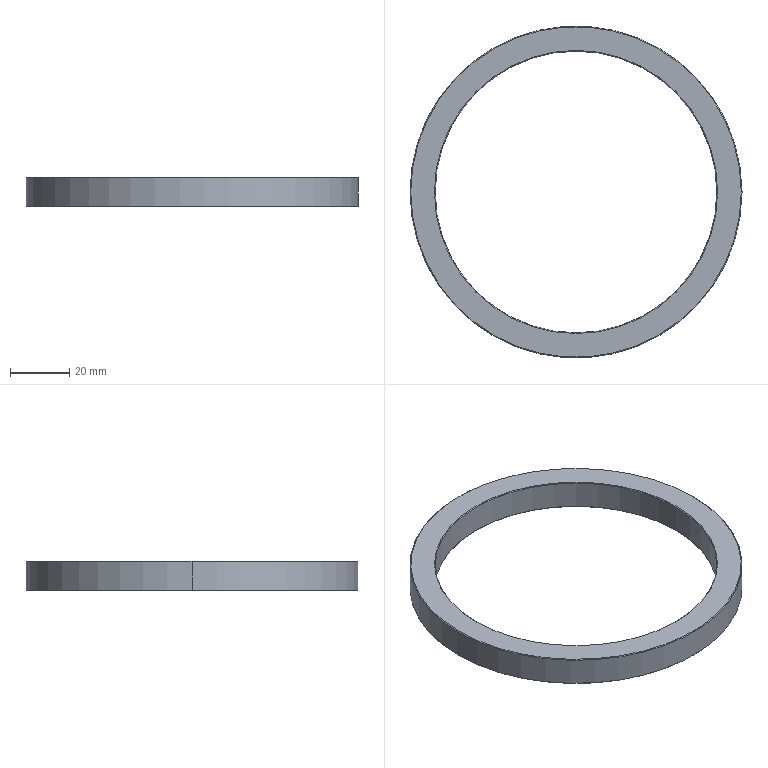Part | SolidWorks | features Chamfer 1, Extrusion 1, HoleWzd 1, ICE 1 | 1 solid | 44 faces | box 112 x 112 x 10 mm | volume 26527 mm3 | cylinder 24 | plane 12 | cone 8 | commonest cylinder face diameters 3.3 x16 95 x2 97 x2 100 x2 112 x2
STEP:
#1=CARTESIAN_POINT('',(-48.5,0.,1.2));
#2=VERTEX_POINT('',#1);
#3=CARTESIAN_POINT('',(48.5,0.,1.2));
#4=VERTEX_POINT('',#3);
#5=CARTESIAN_POINT('',(0.,0.,1.2));
#6=DIRECTION('',(0.,0.,-1.));
#7=DIRECTION('',(-1.,0.,0.));
#8=AXIS2_PLACEMENT_3D('',#5,#6,#7);
#9=CIRCLE('',#8,48.5);
#10=EDGE_CURVE('',#2,#4,#9,.T.);
#11=ORIENTED_EDGE('',*,*,#10,.T.);
#12=CARTESIAN_POINT('',(48.5,0.,0.));
#13=VERTEX_POINT('',#12);
#14=CARTESIAN_POINT('',(48.5,0.,1.2));
#15=DIRECTION('',(0.,0.,-1.));
#16=VECTOR('',#15,1000.);
#17=LINE('',#14,#16);
#18=EDGE_CURVE('',#4,#13,#17,.T.);
#19=ORIENTED_EDGE('',*,*,#18,.T.);
#20=CARTESIAN_POINT('',(-48.5,0.,0.));
#21=VERTEX_POINT('',#20);
#22=CARTESIAN_POINT('',(0.,0.,0.));
#23=DIRECTION('',(0.,0.,-1.));
#24=DIRECTION('',(-1.,0.,0.));
#25=AXIS2_PLACEMENT_3D('',#22,#23,#24);
#26=CIRCLE('',#25,48.5);
#27=EDGE_CURVE('',#21,#13,#26,.T.);
#28=ORIENTED_EDGE('',*,*,#27,.F.);
#29=CARTESIAN_POINT('',(-48.5,0.,1.2));
#30=DIRECTION('',(0.,0.,-1.));
#31=VECTOR('',#30,1000.);
#32=LINE('',#29,#31);
#33=EDGE_CURVE('',#2,#21,#32,.T.);
#34=ORIENTED_EDGE('',*,*,#33,.F.);
#35=EDGE_LOOP('',(#11,#19,#28,#34));
#36=FACE_OUTER_BOUND('',#35,.T.);
#37=CARTESIAN_POINT('',(0.,0.,1.2));
#38=DIRECTION('',(0.,0.,-1.));
#39=DIRECTION('',(-1.,0.,0.));
#40=AXIS2_PLACEMENT_3D('',#37,#38,#39);
#41=CYLINDRICAL_SURFACE('',#40,48.5);
#42=ADVANCED_FACE('',(#36),#41,.T.);
#43=CARTESIAN_POINT('',(50.,0.,1.2));
#44=VERTEX_POINT('',#43);
#45=CARTESIAN_POINT('',(-50.,0.,1.2));
#46=VERTEX_POINT('',#45);
#47=CARTESIAN_POINT('',(0.,0.,1.2));
#48=DIRECTION('',(0.,0.,-1.));
#49=DIRECTION('',(-1.,0.,0.));
#50=AXIS2_PLACEMENT_3D('',#47,#48,#49);
#51=CIRCLE('',#50,50.);
#52=EDGE_CURVE('',#44,#46,#51,.T.);
#53=ORIENTED_EDGE('',*,*,#52,.F.);
#54=CARTESIAN_POINT('',(50.,0.,0.));
#55=VERTEX_POINT('',#54);
#56=CARTESIAN_POINT('',(50.,0.,1.2));
#57=DIRECTION('',(0.,0.,-1.));
#58=VECTOR('',#57,1000.);
#59=LINE('',#56,#58);
#60=EDGE_CURVE('',#44,#55,#59,.T.);
#61=ORIENTED_EDGE('',*,*,#60,.T.);
#62=CARTESIAN_POINT('',(-50.,0.,0.));
#63=VERTEX_POINT('',#62);
#64=CARTESIAN_POINT('',(0.,0.,0.));
#65=DIRECTION('',(0.,0.,-1.));
#66=DIRECTION('',(-1.,0.,0.));
#67=AXIS2_PLACEMENT_3D('',#64,#65,#66);
#68=CIRCLE('',#67,50.);
#69=EDGE_CURVE('',#55,#63,#68,.T.);
#70=ORIENTED_EDGE('',*,*,#69,.T.);
#71=CARTESIAN_POINT('',(-50.,0.,1.2));
#72=DIRECTION('',(0.,0.,-1.));
#73=VECTOR('',#72,1000.);
#74=LINE('',#71,#73);
#75=EDGE_CURVE('',#46,#63,#74,.T.);
#76=ORIENTED_EDGE('',*,*,#75,.F.);
#77=EDGE_LOOP('',(#53,#61,#70,#76));
#78=FACE_OUTER_BOUND('',#77,.T.);
#79=CARTESIAN_POINT('',(0.,0.,1.2));
#80=DIRECTION('',(0.,0.,-1.));
#81=DIRECTION('',(-1.,0.,0.));
#82=AXIS2_PLACEMENT_3D('',#79,#80,#81);
#83=CYLINDRICAL_SURFACE('',#82,50.);
#84=ADVANCED_FACE('',(#78),#83,.F.);
#85=CARTESIAN_POINT('',(47.5,0.,0.25));
#86=VERTEX_POINT('',#85);
#87=CARTESIAN_POINT('',(-47.5,0.,0.25));
#88=VERTEX_POINT('',#87);
#89=CARTESIAN_POINT('',(0.,0.,0.25));
#90=DIRECTION('',(0.,0.,-1.));
#91=DIRECTION('',(1.,0.,0.));
#92=AXIS2_PLACEMENT_3D('',#89,#90,#91);
#93=CIRCLE('',#92,47.5);
#94=EDGE_CURVE('',#86,#88,#93,.T.);
#95=ORIENTED_EDGE('',*,*,#94,.F.);
#96=CARTESIAN_POINT('',(47.75,0.,0.));
#97=VERTEX_POINT('',#96);
#98=CARTESIAN_POINT('',(47.75,0.,0.));
#99=DIRECTION('',(0.7071,0.,-0.7071));
#100=VECTOR('',#99,1000.);
#101=LINE('',#98,#100);
#102=EDGE_CURVE('',#86,#97,#101,.T.);
#103=ORIENTED_EDGE('',*,*,#102,.T.);
#104=CARTESIAN_POINT('',(-47.75,0.,0.));
#105=VERTEX_POINT('',#104);
#106=CARTESIAN_POINT('',(0.,0.,0.));
#107=DIRECTION('',(0.,0.,1.));
#108=DIRECTION('',(1.,0.,0.));
#109=AXIS2_PLACEMENT_3D('',#106,#107,#108);
#110=CIRCLE('',#109,47.75);
#111=EDGE_CURVE('',#105,#97,#110,.T.);
#112=ORIENTED_EDGE('',*,*,#111,.F.);
#113=CARTESIAN_POINT('',(-47.75,0.,0.));
#114=DIRECTION('',(-0.7071,0.,-0.7071));
#115=VECTOR('',#114,1000.);
#116=LINE('',#113,#115);
#117=EDGE_CURVE('',#88,#105,#116,.T.);
#118=ORIENTED_EDGE('',*,*,#117,.F.);
#119=EDGE_LOOP('',(#95,#103,#112,#118));
#120=FACE_OUTER_BOUND('',#119,.T.);
#121=CARTESIAN_POINT('',(0.,0.,0.));
#122=DIRECTION('',(0.,0.,-1.));
#123=DIRECTION('',(-1.,0.,0.));
#124=AXIS2_PLACEMENT_3D('',#121,#122,#123);
#125=CONICAL_SURFACE('',#124,47.75,0.7854);
#126=ADVANCED_FACE('',(#120),#125,.F.);
#127=CARTESIAN_POINT('',(-55.75,0.,0.));
#128=VERTEX_POINT('',#127);
#129=CARTESIAN_POINT('',(55.75,0.,0.));
#130=VERTEX_POINT('',#129);
#131=CARTESIAN_POINT('',(0.,0.,0.));
#132=DIRECTION('',(0.,0.,-1.));
#133=DIRECTION('',(1.,0.,0.));
#134=AXIS2_PLACEMENT_3D('',#131,#132,#133);
#135=CIRCLE('',#134,55.75);
#136=EDGE_CURVE('',#128,#130,#135,.T.);
#137=ORIENTED_EDGE('',*,*,#136,.F.);
#138=CARTESIAN_POINT('',(-56.,0.,0.25));
#139=VERTEX_POINT('',#138);
#140=CARTESIAN_POINT('',(-56.,0.,0.25));
#141=DIRECTION('',(-0.7071,0.,0.7071));
#142=VECTOR('',#141,1000.);
#143=LINE('',#140,#142);
#144=EDGE_CURVE('',#128,#139,#143,.T.);
#145=ORIENTED_EDGE('',*,*,#144,.T.);
#146=CARTESIAN_POINT('',(56.,0.,0.25));
#147=VERTEX_POINT('',#146);
#148=CARTESIAN_POINT('',(0.,0.,0.25));
#149=DIRECTION('',(0.,0.,1.));
#150=DIRECTION('',(1.,0.,0.));
#151=AXIS2_PLACEMENT_3D('',#148,#149,#150);
#152=CIRCLE('',#151,56.);
#153=EDGE_CURVE('',#147,#139,#152,.T.);
#154=ORIENTED_EDGE('',*,*,#153,.F.);
#155=CARTESIAN_POINT('',(56.,0.,0.25));
#156=DIRECTION('',(0.7071,0.,0.7071));
#157=VECTOR('',#156,1000.);
#158=LINE('',#155,#157);
#159=EDGE_CURVE('',#130,#147,#158,.T.);
#160=ORIENTED_EDGE('',*,*,#159,.F.);
#161=EDGE_LOOP('',(#137,#145,#154,#160));
#162=FACE_OUTER_BOUND('',#161,.T.);
#163=CARTESIAN_POINT('',(0.,0.,0.25));
#164=DIRECTION('',(0.,0.,1.));
#165=DIRECTION('',(1.,0.,0.));
#166=AXIS2_PLACEMENT_3D('',#163,#164,#165);
#167=CONICAL_SURFACE('',#166,56.,0.7854);
#168=ADVANCED_FACE('',(#162),#167,.T.);
#169=CARTESIAN_POINT('',(-47.5,0.,9.75));
#170=VERTEX_POINT('',#169);
#171=CARTESIAN_POINT('',(47.5,0.,9.75));
#172=VERTEX_POINT('',#171);
#173=CARTESIAN_POINT('',(0.,0.,9.75));
#174=DIRECTION('',(0.,0.,1.));
#175=DIRECTION('',(1.,0.,0.));
#176=AXIS2_PLACEMENT_3D('',#173,#174,#175);
#177=CIRCLE('',#176,47.5);
#178=EDGE_CURVE('',#170,#172,#177,.T.);
#179=ORIENTED_EDGE('',*,*,#178,.F.);
#180=CARTESIAN_POINT('',(-47.75,0.,10.));
#181=VERTEX_POINT('',#180);
#182=CARTESIAN_POINT('',(-47.5,0.,9.75));
#183=DIRECTION('',(-0.7071,0.,0.7071));
#184=VECTOR('',#183,1000.);
#185=LINE('',#182,#184);
#186=EDGE_CURVE('',#170,#181,#185,.T.);
#187=ORIENTED_EDGE('',*,*,#186,.T.);
#188=CARTESIAN_POINT('',(47.75,0.,10.));
#189=VERTEX_POINT('',#188);
#190=CARTESIAN_POINT('',(0.,0.,10.));
#191=DIRECTION('',(0.,0.,-1.));
#192=DIRECTION('',(1.,0.,0.));
#193=AXIS2_PLACEMENT_3D('',#190,#191,#192);
#194=CIRCLE('',#193,47.75);
#195=EDGE_CURVE('',#189,#181,#194,.T.);
#196=ORIENTED_EDGE('',*,*,#195,.F.);
#197=CARTESIAN_POINT('',(47.5,0.,9.75));
#198=DIRECTION('',(0.7071,0.,0.7071));
#199=VECTOR('',#198,1000.);
#200=LINE('',#197,#199);
#201=EDGE_CURVE('',#172,#189,#200,.T.);
#202=ORIENTED_EDGE('',*,*,#201,.F.);
#203=EDGE_LOOP('',(#179,#187,#196,#202));
#204=FACE_OUTER_BOUND('',#203,.T.);
#205=CARTESIAN_POINT('',(0.,0.,9.75));
#206=DIRECTION('',(0.,0.,1.));
#207=DIRECTION('',(1.,0.,0.));
#208=AXIS2_PLACEMENT_3D('',#205,#206,#207);
#209=CONICAL_SURFACE('',#208,47.5,0.7854);
#210=ADVANCED_FACE('',(#204),#209,.F.);
#211=CARTESIAN_POINT('',(55.75,0.,10.));
#212=VERTEX_POINT('',#211);
#213=CARTESIAN_POINT('',(-55.75,0.,10.));
#214=VERTEX_POINT('',#213);
#215=CARTESIAN_POINT('',(0.,0.,10.));
#216=DIRECTION('',(0.,0.,1.));
#217=DIRECTION('',(1.,0.,0.));
#218=AXIS2_PLACEMENT_3D('',#215,#216,#217);
#219=CIRCLE('',#218,55.75);
#220=EDGE_CURVE('',#212,#214,#219,.T.);
#221=ORIENTED_EDGE('',*,*,#220,.F.);
#222=CARTESIAN_POINT('',(56.,0.,9.75));
#223=VERTEX_POINT('',#222);
#224=CARTESIAN_POINT('',(55.75,0.,10.));
#225=DIRECTION('',(0.7071,0.,-0.7071));
#226=VECTOR('',#225,1000.);
#227=LINE('',#224,#226);
#228=EDGE_CURVE('',#212,#223,#227,.T.);
#229=ORIENTED_EDGE('',*,*,#228,.T.);
#230=CARTESIAN_POINT('',(-56.,0.,9.75));
#231=VERTEX_POINT('',#230);
#232=CARTESIAN_POINT('',(0.,0.,9.75));
#233=DIRECTION('',(0.,0.,-1.));
#234=DIRECTION('',(1.,0.,0.));
#235=AXIS2_PLACEMENT_3D('',#232,#233,#234);
#236=CIRCLE('',#235,56.);
#237=EDGE_CURVE('',#231,#223,#236,.T.);
#238=ORIENTED_EDGE('',*,*,#237,.F.);
#239=CARTESIAN_POINT('',(-55.75,0.,10.));
#240=DIRECTION('',(-0.7071,0.,-0.7071));
#241=VECTOR('',#240,1000.);
#242=LINE('',#239,#241);
#243=EDGE_CURVE('',#214,#231,#242,.T.);
#244=ORIENTED_EDGE('',*,*,#243,.F.);
#245=EDGE_LOOP('',(#221,#229,#238,#244));
#246=FACE_OUTER_BOUND('',#245,.T.);
#247=CARTESIAN_POINT('',(0.,0.,10.));
#248=DIRECTION('',(0.,0.,-1.));
#249=DIRECTION('',(-1.,0.,0.));
#250=AXIS2_PLACEMENT_3D('',#247,#248,#249);
#251=CONICAL_SURFACE('',#250,55.75,0.7854);
#252=ADVANCED_FACE('',(#246),#251,.T.);
#253=CARTESIAN_POINT('',(39.127,-37.477,7.5));
#254=VERTEX_POINT('',#253);
#255=CARTESIAN_POINT('',(35.827,-37.477,7.5));
#256=VERTEX_POINT('',#255);
#257=CARTESIAN_POINT('',(37.477,-37.477,7.5));
#258=DIRECTION('',(0.,0.,-1.));
#259=DIRECTION('',(-1.,0.,0.));
#260=AXIS2_PLACEMENT_3D('',#257,#258,#259);
#261=CIRCLE('',#260,1.65);
#262=EDGE_CURVE('',#254,#256,#261,.T.);
#263=ORIENTED_EDGE('',*,*,#262,.F.);
#264=CARTESIAN_POINT('',(39.127,-37.477,0.));
#265=VERTEX_POINT('',#264);
#266=CARTESIAN_POINT('',(39.127,-37.477,0.));
#267=DIRECTION('',(0.,0.,-1.));
#268=VECTOR('',#267,1000.);
#269=LINE('',#266,#268);
#270=EDGE_CURVE('',#254,#265,#269,.T.);
#271=ORIENTED_EDGE('',*,*,#270,.T.);
#272=CARTESIAN_POINT('',(35.827,-37.477,0.));
#273=VERTEX_POINT('',#272);
#274=CARTESIAN_POINT('',(37.477,-37.477,0.));
#275=DIRECTION('',(0.,0.,-1.));
#276=DIRECTION('',(-1.,0.,0.));
#277=AXIS2_PLACEMENT_3D('',#274,#275,#276);
#278=CIRCLE('',#277,1.65);
#279=EDGE_CURVE('',#265,#273,#278,.T.);
#280=ORIENTED_EDGE('',*,*,#279,.T.);
#281=CARTESIAN_POINT('',(35.827,-37.477,0.));
#282=DIRECTION('',(0.,0.,-1.));
#283=VECTOR('',#282,1000.);
#284=LINE('',#281,#283);
#285=EDGE_CURVE('',#256,#273,#284,.T.);
#286=ORIENTED_EDGE('',*,*,#285,.F.);
#287=EDGE_LOOP('',(#263,#271,#280,#286));
#288=FACE_OUTER_BOUND('',#287,.T.);
#289=CARTESIAN_POINT('',(37.477,-37.477,0.));
#290=DIRECTION('',(0.,0.,-1.));
#291=DIRECTION('',(-1.,0.,0.));
#292=AXIS2_PLACEMENT_3D('',#289,#290,#291);
#293=CYLINDRICAL_SURFACE('',#292,1.65);
#294=ADVANCED_FACE('',(#288),#293,.F.);
#295=CARTESIAN_POINT('',(-35.827,-37.477,7.5));
#296=VERTEX_POINT('',#295);
#297=CARTESIAN_POINT('',(-39.127,-37.477,7.5));
#298=VERTEX_POINT('',#297);
#299=CARTESIAN_POINT('',(-37.477,-37.477,7.5));
#300=DIRECTION('',(0.,0.,-1.));
#301=DIRECTION('',(-1.,0.,0.));
#302=AXIS2_PLACEMENT_3D('',#299,#300,#301);
#303=CIRCLE('',#302,1.65);
#304=EDGE_CURVE('',#296,#298,#303,.T.);
#305=ORIENTED_EDGE('',*,*,#304,.F.);
#306=CARTESIAN_POINT('',(-35.827,-37.477,0.));
#307=VERTEX_POINT('',#306);
#308=CARTESIAN_POINT('',(-35.827,-37.477,0.));
#309=DIRECTION('',(0.,0.,-1.));
#310=VECTOR('',#309,1000.);
#311=LINE('',#308,#310);
#312=EDGE_CURVE('',#296,#307,#311,.T.);
#313=ORIENTED_EDGE('',*,*,#312,.T.);
#314=CARTESIAN_POINT('',(-39.127,-37.477,0.));
#315=VERTEX_POINT('',#314);
#316=CARTESIAN_POINT('',(-37.477,-37.477,0.));
#317=DIRECTION('',(0.,0.,-1.));
#318=DIRECTION('',(-1.,0.,0.));
#319=AXIS2_PLACEMENT_3D('',#316,#317,#318);
#320=CIRCLE('',#319,1.65);
#321=EDGE_CURVE('',#307,#315,#320,.T.);
#322=ORIENTED_EDGE('',*,*,#321,.T.);
#323=CARTESIAN_POINT('',(-39.127,-37.477,0.));
#324=DIRECTION('',(0.,0.,-1.));
#325=VECTOR('',#324,1000.);
#326=LINE('',#323,#325);
#327=EDGE_CURVE('',#298,#315,#326,.T.);
#328=ORIENTED_EDGE('',*,*,#327,.F.);
#329=EDGE_LOOP('',(#305,#313,#322,#328));
#330=FACE_OUTER_BOUND('',#329,.T.);
#331=CARTESIAN_POINT('',(-37.477,-37.477,0.));
#332=DIRECTION('',(0.,0.,-1.));
#333=DIRECTION('',(-1.,0.,0.));
#334=AXIS2_PLACEMENT_3D('',#331,#332,#333);
#335=CYLINDRICAL_SURFACE('',#334,1.65);
#336=ADVANCED_FACE('',(#330),#335,.F.);
#337=CARTESIAN_POINT('',(-35.827,37.477,7.5));
#338=VERTEX_POINT('',#337);
#339=CARTESIAN_POINT('',(-39.127,37.477,7.5));
#340=VERTEX_POINT('',#339);
#341=CARTESIAN_POINT('',(-37.477,37.477,7.5));
#342=DIRECTION('',(0.,0.,-1.));
#343=DIRECTION('',(-1.,0.,0.));
#344=AXIS2_PLACEMENT_3D('',#341,#342,#343);
#345=CIRCLE('',#344,1.65);
#346=EDGE_CURVE('',#338,#340,#345,.T.);
#347=ORIENTED_EDGE('',*,*,#346,.F.);
#348=CARTESIAN_POINT('',(-35.827,37.477,0.));
#349=VERTEX_POINT('',#348);
#350=CARTESIAN_POINT('',(-35.827,37.477,0.));
#351=DIRECTION('',(0.,0.,-1.));
#352=VECTOR('',#351,1000.);
#353=LINE('',#350,#352);
#354=EDGE_CURVE('',#338,#349,#353,.T.);
#355=ORIENTED_EDGE('',*,*,#354,.T.);
#356=CARTESIAN_POINT('',(-39.127,37.477,0.));
#357=VERTEX_POINT('',#356);
#358=CARTESIAN_POINT('',(-37.477,37.477,0.));
#359=DIRECTION('',(0.,0.,-1.));
#360=DIRECTION('',(-1.,0.,0.));
#361=AXIS2_PLACEMENT_3D('',#358,#359,#360);
#362=CIRCLE('',#361,1.65);
#363=EDGE_CURVE('',#349,#357,#362,.T.);
#364=ORIENTED_EDGE('',*,*,#363,.T.);
#365=CARTESIAN_POINT('',(-39.127,37.477,0.));
#366=DIRECTION('',(0.,0.,-1.));
#367=VECTOR('',#366,1000.);
#368=LINE('',#365,#367);
#369=EDGE_CURVE('',#340,#357,#368,.T.);
#370=ORIENTED_EDGE('',*,*,#369,.F.);
#371=EDGE_LOOP('',(#347,#355,#364,#370));
#372=FACE_OUTER_BOUND('',#371,.T.);
#373=CARTESIAN_POINT('',(-37.477,37.477,0.));
#374=DIRECTION('',(0.,0.,-1.));
#375=DIRECTION('',(-1.,0.,0.));
#376=AXIS2_PLACEMENT_3D('',#373,#374,#375);
#377=CYLINDRICAL_SURFACE('',#376,1.65);
#378=ADVANCED_FACE('',(#372),#377,.F.);
#379=CARTESIAN_POINT('',(39.127,37.477,7.5));
#380=VERTEX_POINT('',#379);
#381=CARTESIAN_POINT('',(35.827,37.477,7.5));
#382=VERTEX_POINT('',#381);
#383=CARTESIAN_POINT('',(37.477,37.477,7.5));
#384=DIRECTION('',(0.,0.,-1.));
#385=DIRECTION('',(-1.,0.,0.));
#386=AXIS2_PLACEMENT_3D('',#383,#384,#385);
#387=CIRCLE('',#386,1.65);
#388=EDGE_CURVE('',#380,#382,#387,.T.);
#389=ORIENTED_EDGE('',*,*,#388,.F.);
#390=CARTESIAN_POINT('',(39.127,37.477,0.));
#391=VERTEX_POINT('',#390);
#392=CARTESIAN_POINT('',(39.127,37.477,0.));
#393=DIRECTION('',(0.,0.,-1.));
#394=VECTOR('',#393,1000.);
#395=LINE('',#392,#394);
#396=EDGE_CURVE('',#380,#391,#395,.T.);
#397=ORIENTED_EDGE('',*,*,#396,.T.);
#398=CARTESIAN_POINT('',(35.827,37.477,0.));
#399=VERTEX_POINT('',#398);
#400=CARTESIAN_POINT('',(37.477,37.477,0.));
#401=DIRECTION('',(0.,0.,-1.));
#402=DIRECTION('',(-1.,0.,0.));
#403=AXIS2_PLACEMENT_3D('',#400,#401,#402);
#404=CIRCLE('',#403,1.65);
#405=EDGE_CURVE('',#391,#399,#404,.T.);
#406=ORIENTED_EDGE('',*,*,#405,.T.);
#407=CARTESIAN_POINT('',(35.827,37.477,0.));
#408=DIRECTION('',(0.,0.,-1.));
#409=VECTOR('',#408,1000.);
#410=LINE('',#407,#409);
#411=EDGE_CURVE('',#382,#399,#410,.T.);
#412=ORIENTED_EDGE('',*,*,#411,.F.);
#413=EDGE_LOOP('',(#389,#397,#406,#412));
#414=FACE_OUTER_BOUND('',#413,.T.);
#415=CARTESIAN_POINT('',(37.477,37.477,0.));
#416=DIRECTION('',(0.,0.,-1.));
#417=DIRECTION('',(-1.,0.,0.));
#418=AXIS2_PLACEMENT_3D('',#415,#416,#417);
#419=CYLINDRICAL_SURFACE('',#418,1.65);
#420=ADVANCED_FACE('',(#414),#419,.F.);
#421=CARTESIAN_POINT('',(1.65,53.,7.5));
#422=VERTEX_POINT('',#421);
#423=CARTESIAN_POINT('',(-1.65,53.,7.5));
#424=VERTEX_POINT('',#423);
#425=CARTESIAN_POINT('',(0.,53.,7.5));
#426=DIRECTION('',(0.,0.,-1.));
#427=DIRECTION('',(-1.,0.,0.));
#428=AXIS2_PLACEMENT_3D('',#425,#426,#427);
#429=CIRCLE('',#428,1.65);
#430=EDGE_CURVE('',#422,#424,#429,.T.);
#431=ORIENTED_EDGE('',*,*,#430,.F.);
#432=CARTESIAN_POINT('',(1.65,53.,0.));
#433=VERTEX_POINT('',#432);
#434=CARTESIAN_POINT('',(1.65,53.,0.));
#435=DIRECTION('',(0.,0.,-1.));
#436=VECTOR('',#435,1000.);
#437=LINE('',#434,#436);
#438=EDGE_CURVE('',#422,#433,#437,.T.);
#439=ORIENTED_EDGE('',*,*,#438,.T.);
#440=CARTESIAN_POINT('',(-1.65,53.,0.));
#441=VERTEX_POINT('',#440);
#442=CARTESIAN_POINT('',(0.,53.,0.));
#443=DIRECTION('',(0.,0.,-1.));
#444=DIRECTION('',(-1.,0.,0.));
#445=AXIS2_PLACEMENT_3D('',#442,#443,#444);
#446=CIRCLE('',#445,1.65);
#447=EDGE_CURVE('',#433,#441,#446,.T.);
#448=ORIENTED_EDGE('',*,*,#447,.T.);
#449=CARTESIAN_POINT('',(-1.65,53.,0.));
#450=DIRECTION('',(0.,0.,-1.));
#451=VECTOR('',#450,1000.);
#452=LINE('',#449,#451);
#453=EDGE_CURVE('',#424,#441,#452,.T.);
#454=ORIENTED_EDGE('',*,*,#453,.F.);
#455=EDGE_LOOP('',(#431,#439,#448,#454));
#456=FACE_OUTER_BOUND('',#455,.T.);
#457=CARTESIAN_POINT('',(0.,53.,0.));
#458=DIRECTION('',(0.,0.,-1.));
#459=DIRECTION('',(-1.,0.,0.));
#460=AXIS2_PLACEMENT_3D('',#457,#458,#459);
#461=CYLINDRICAL_SURFACE('',#460,1.65);
#462=ADVANCED_FACE('',(#456),#461,.F.);
#463=CARTESIAN_POINT('',(-51.35,0.,7.5));
#464=VERTEX_POINT('',#463);
#465=CARTESIAN_POINT('',(-54.65,0.,7.5));
#466=VERTEX_POINT('',#465);
#467=CARTESIAN_POINT('',(-53.,0.,7.5));
#468=DIRECTION('',(0.,0.,-1.));
#469=DIRECTION('',(-1.,0.,0.));
#470=AXIS2_PLACEMENT_3D('',#467,#468,#469);
#471=CIRCLE('',#470,1.65);
#472=EDGE_CURVE('',#464,#466,#471,.T.);
#473=ORIENTED_EDGE('',*,*,#472,.F.);
#474=CARTESIAN_POINT('',(-51.35,0.,0.));
#475=VERTEX_POINT('',#474);
#476=CARTESIAN_POINT('',(-51.35,0.,0.));
#477=DIRECTION('',(0.,0.,-1.));
#478=VECTOR('',#477,1000.);
#479=LINE('',#476,#478);
#480=EDGE_CURVE('',#464,#475,#479,.T.);
#481=ORIENTED_EDGE('',*,*,#480,.T.);
#482=CARTESIAN_POINT('',(-54.65,0.,0.));
#483=VERTEX_POINT('',#482);
#484=CARTESIAN_POINT('',(-53.,0.,0.));
#485=DIRECTION('',(0.,0.,-1.));
#486=DIRECTION('',(-1.,0.,0.));
#487=AXIS2_PLACEMENT_3D('',#484,#485,#486);
#488=CIRCLE('',#487,1.65);
#489=EDGE_CURVE('',#475,#483,#488,.T.);
#490=ORIENTED_EDGE('',*,*,#489,.T.);
#491=CARTESIAN_POINT('',(-54.65,0.,0.));
#492=DIRECTION('',(0.,0.,-1.));
#493=VECTOR('',#492,1000.);
#494=LINE('',#491,#493);
#495=EDGE_CURVE('',#466,#483,#494,.T.);
#496=ORIENTED_EDGE('',*,*,#495,.F.);
#497=EDGE_LOOP('',(#473,#481,#490,#496));
#498=FACE_OUTER_BOUND('',#497,.T.);
#499=CARTESIAN_POINT('',(-53.,0.,0.));
#500=DIRECTION('',(0.,0.,-1.));
#501=DIRECTION('',(-1.,0.,0.));
#502=AXIS2_PLACEMENT_3D('',#499,#500,#501);
#503=CYLINDRICAL_SURFACE('',#502,1.65);
#504=ADVANCED_FACE('',(#498),#503,.F.);
#505=CARTESIAN_POINT('',(1.65,-53.,7.5));
#506=VERTEX_POINT('',#505);
#507=CARTESIAN_POINT('',(-1.65,-53.,7.5));
#508=VERTEX_POINT('',#507);
#509=CARTESIAN_POINT('',(0.,-53.,7.5));
#510=DIRECTION('',(0.,0.,-1.));
#511=DIRECTION('',(-1.,0.,0.));
#512=AXIS2_PLACEMENT_3D('',#509,#510,#511);
#513=CIRCLE('',#512,1.65);
#514=EDGE_CURVE('',#506,#508,#513,.T.);
#515=ORIENTED_EDGE('',*,*,#514,.F.);
#516=CARTESIAN_POINT('',(1.65,-53.,0.));
#517=VERTEX_POINT('',#516);
#518=CARTESIAN_POINT('',(1.65,-53.,0.));
#519=DIRECTION('',(0.,0.,-1.));
#520=VECTOR('',#519,1000.);
#521=LINE('',#518,#520);
#522=EDGE_CURVE('',#506,#517,#521,.T.);
#523=ORIENTED_EDGE('',*,*,#522,.T.);
#524=CARTESIAN_POINT('',(-1.65,-53.,0.));
#525=VERTEX_POINT('',#524);
#526=CARTESIAN_POINT('',(0.,-53.,0.));
#527=DIRECTION('',(0.,0.,-1.));
#528=DIRECTION('',(-1.,0.,0.));
#529=AXIS2_PLACEMENT_3D('',#526,#527,#528);
#530=CIRCLE('',#529,1.65);
#531=EDGE_CURVE('',#517,#525,#530,.T.);
#532=ORIENTED_EDGE('',*,*,#531,.T.);
#533=CARTESIAN_POINT('',(-1.65,-53.,0.));
#534=DIRECTION('',(0.,0.,-1.));
#535=VECTOR('',#534,1000.);
#536=LINE('',#533,#535);
#537=EDGE_CURVE('',#508,#525,#536,.T.);
#538=ORIENTED_EDGE('',*,*,#537,.F.);
#539=EDGE_LOOP('',(#515,#523,#532,#538));
#540=FACE_OUTER_BOUND('',#539,.T.);
#541=CARTESIAN_POINT('',(0.,-53.,0.));
#542=DIRECTION('',(0.,0.,-1.));
#543=DIRECTION('',(-1.,0.,0.));
#544=AXIS2_PLACEMENT_3D('',#541,#542,#543);
#545=CYLINDRICAL_SURFACE('',#544,1.65);
#546=ADVANCED_FACE('',(#540),#545,.F.);
#547=CARTESIAN_POINT('',(54.65,0.,7.5));
#548=VERTEX_POINT('',#547);
#549=CARTESIAN_POINT('',(51.35,0.,7.5));
#550=VERTEX_POINT('',#549);
#551=CARTESIAN_POINT('',(53.,0.,7.5));
#552=DIRECTION('',(0.,0.,-1.));
#553=DIRECTION('',(-1.,0.,0.));
#554=AXIS2_PLACEMENT_3D('',#551,#552,#553);
#555=CIRCLE('',#554,1.65);
#556=EDGE_CURVE('',#548,#550,#555,.T.);
#557=ORIENTED_EDGE('',*,*,#556,.F.);
#558=CARTESIAN_POINT('',(54.65,0.,0.));
#559=VERTEX_POINT('',#558);
#560=CARTESIAN_POINT('',(54.65,0.,0.));
#561=DIRECTION('',(0.,0.,-1.));
#562=VECTOR('',#561,1000.);
#563=LINE('',#560,#562);
#564=EDGE_CURVE('',#548,#559,#563,.T.);
#565=ORIENTED_EDGE('',*,*,#564,.T.);
#566=CARTESIAN_POINT('',(51.35,0.,0.));
#567=VERTEX_POINT('',#566);
#568=CARTESIAN_POINT('',(53.,0.,0.));
#569=DIRECTION('',(0.,0.,-1.));
#570=DIRECTION('',(-1.,0.,0.));
#571=AXIS2_PLACEMENT_3D('',#568,#569,#570);
#572=CIRCLE('',#571,1.65);
#573=EDGE_CURVE('',#559,#567,#572,.T.);
#574=ORIENTED_EDGE('',*,*,#573,.T.);
#575=CARTESIAN_POINT('',(51.35,0.,0.));
#576=DIRECTION('',(0.,0.,-1.));
#577=VECTOR('',#576,1000.);
#578=LINE('',#575,#577);
#579=EDGE_CURVE('',#550,#567,#578,.T.);
#580=ORIENTED_EDGE('',*,*,#579,.F.);
#581=EDGE_LOOP('',(#557,#565,#574,#580));
#582=FACE_OUTER_BOUND('',#581,.T.);
#583=CARTESIAN_POINT('',(53.,0.,0.));
#584=DIRECTION('',(0.,0.,-1.));
#585=DIRECTION('',(-1.,0.,0.));
#586=AXIS2_PLACEMENT_3D('',#583,#584,#585);
#587=CYLINDRICAL_SURFACE('',#586,1.65);
#588=ADVANCED_FACE('',(#582),#587,.F.);
#589=ORIENTED_EDGE('',*,*,#178,.T.);
#590=CARTESIAN_POINT('',(47.5,0.,10.));
#591=DIRECTION('',(0.,0.,-1.));
#592=VECTOR('',#591,1000.);
#593=LINE('',#590,#592);
#594=EDGE_CURVE('',#172,#86,#593,.T.);
#595=ORIENTED_EDGE('',*,*,#594,.T.);
#596=ORIENTED_EDGE('',*,*,#94,.T.);
#597=CARTESIAN_POINT('',(-47.5,0.,10.));
#598=DIRECTION('',(0.,0.,-1.));
#599=VECTOR('',#598,1000.);
#600=LINE('',#597,#599);
#601=EDGE_CURVE('',#170,#88,#600,.T.);
#602=ORIENTED_EDGE('',*,*,#601,.F.);
#603=EDGE_LOOP('',(#589,#595,#596,#602));
#604=FACE_OUTER_BOUND('',#603,.T.);
#605=CARTESIAN_POINT('',(0.,0.,10.));
#606=DIRECTION('',(0.,0.,-1.));
#607=DIRECTION('',(-1.,0.,0.));
#608=AXIS2_PLACEMENT_3D('',#605,#606,#607);
#609=CYLINDRICAL_SURFACE('',#608,47.5);
#610=ADVANCED_FACE('',(#604),#609,.F.);
#611=ORIENTED_EDGE('',*,*,#237,.T.);
#612=CARTESIAN_POINT('',(56.,0.,10.));
#613=DIRECTION('',(0.,0.,-1.));
#614=VECTOR('',#613,1000.);
#615=LINE('',#612,#614);
#616=EDGE_CURVE('',#223,#147,#615,.T.);
#617=ORIENTED_EDGE('',*,*,#616,.T.);
#618=ORIENTED_EDGE('',*,*,#153,.T.);
#619=CARTESIAN_POINT('',(-56.,0.,10.));
#620=DIRECTION('',(0.,0.,-1.));
#621=VECTOR('',#620,1000.);
#622=LINE('',#619,#621);
#623=EDGE_CURVE('',#231,#139,#622,.T.);
#624=ORIENTED_EDGE('',*,*,#623,.F.);
#625=EDGE_LOOP('',(#611,#617,#618,#624));
#626=FACE_OUTER_BOUND('',#625,.T.);
#627=CARTESIAN_POINT('',(0.,0.,10.));
#628=DIRECTION('',(0.,0.,-1.));
#629=DIRECTION('',(-1.,0.,0.));
#630=AXIS2_PLACEMENT_3D('',#627,#628,#629);
#631=CYLINDRICAL_SURFACE('',#630,56.);
#632=ADVANCED_FACE('',(#626),#631,.T.);
#633=ORIENTED_EDGE('',*,*,#111,.T.);
#634=CARTESIAN_POINT('',(0.,0.,0.));
#635=DIRECTION('',(0.,0.,1.));
#636=DIRECTION('',(1.,0.,0.));
#637=AXIS2_PLACEMENT_3D('',#634,#635,#636);
#638=CIRCLE('',#637,47.75);
#639=EDGE_CURVE('',#97,#105,#638,.T.);
#640=ORIENTED_EDGE('',*,*,#639,.T.);
#641=EDGE_LOOP('',(#633,#640));
#642=FACE_BOUND('',#641,.T.);
#643=ORIENTED_EDGE('',*,*,#27,.T.);
#644=CARTESIAN_POINT('',(0.,0.,0.));
#645=DIRECTION('',(0.,0.,-1.));
#646=DIRECTION('',(-1.,0.,0.));
#647=AXIS2_PLACEMENT_3D('',#644,#645,#646);
#648=CIRCLE('',#647,48.5);
#649=EDGE_CURVE('',#13,#21,#648,.T.);
#650=ORIENTED_EDGE('',*,*,#649,.T.);
#651=EDGE_LOOP('',(#643,#650));
#652=FACE_OUTER_BOUND('',#651,.T.);
#653=CARTESIAN_POINT('',(0.,0.,0.));
#654=DIRECTION('',(0.,0.,1.));
#655=DIRECTION('',(1.,0.,0.));
#656=AXIS2_PLACEMENT_3D('',#653,#654,#655);
#657=PLANE('',#656);
#658=ADVANCED_FACE('',(#642,#652),#657,.F.);
#659=CARTESIAN_POINT('',(0.,0.,10.));
#660=DIRECTION('',(0.,0.,1.));
#661=DIRECTION('',(1.,0.,0.));
#662=AXIS2_PLACEMENT_3D('',#659,#660,#661);
#663=CIRCLE('',#662,55.75);
#664=EDGE_CURVE('',#214,#212,#663,.T.);
#665=ORIENTED_EDGE('',*,*,#664,.T.);
#666=ORIENTED_EDGE('',*,*,#220,.T.);
#667=EDGE_LOOP('',(#665,#666));
#668=FACE_OUTER_BOUND('',#667,.T.);
#669=ORIENTED_EDGE('',*,*,#195,.T.);
#670=CARTESIAN_POINT('',(0.,0.,10.));
#671=DIRECTION('',(0.,0.,-1.));
#672=DIRECTION('',(1.,0.,0.));
#673=AXIS2_PLACEMENT_3D('',#670,#671,#672);
#674=CIRCLE('',#673,47.75);
#675=EDGE_CURVE('',#181,#189,#674,.T.);
#676=ORIENTED_EDGE('',*,*,#675,.T.);
#677=EDGE_LOOP('',(#669,#676));
#678=FACE_BOUND('',#677,.T.);
#679=CARTESIAN_POINT('',(0.,0.,10.));
#680=DIRECTION('',(0.,0.,1.));
#681=DIRECTION('',(1.,0.,0.));
#682=AXIS2_PLACEMENT_3D('',#679,#680,#681);
#683=PLANE('',#682);
#684=ADVANCED_FACE('',(#668,#678),#683,.T.);
#685=CARTESIAN_POINT('',(0.,0.,0.));
#686=DIRECTION('',(0.,0.,-1.));
#687=DIRECTION('',(-1.,0.,0.));
#688=AXIS2_PLACEMENT_3D('',#685,#686,#687);
#689=CIRCLE('',#688,50.);
#690=EDGE_CURVE('',#63,#55,#689,.T.);
#691=ORIENTED_EDGE('',*,*,#690,.F.);
#692=ORIENTED_EDGE('',*,*,#69,.F.);
#693=EDGE_LOOP('',(#691,#692));
#694=FACE_BOUND('',#693,.T.);
#695=CARTESIAN_POINT('',(0.,0.,0.));
#696=DIRECTION('',(0.,0.,-1.));
#697=DIRECTION('',(1.,0.,0.));
#698=AXIS2_PLACEMENT_3D('',#695,#696,#697);
#699=CIRCLE('',#698,55.75);
#700=EDGE_CURVE('',#130,#128,#699,.T.);
#701=ORIENTED_EDGE('',*,*,#700,.T.);
#702=ORIENTED_EDGE('',*,*,#136,.T.);
#703=EDGE_LOOP('',(#701,#702));
#704=FACE_OUTER_BOUND('',#703,.T.);
#705=CARTESIAN_POINT('',(37.477,-37.477,0.));
#706=DIRECTION('',(0.,0.,-1.));
#707=DIRECTION('',(-1.,0.,0.));
#708=AXIS2_PLACEMENT_3D('',#705,#706,#707);
#709=CIRCLE('',#708,1.65);
#710=EDGE_CURVE('',#273,#265,#709,.T.);
#711=ORIENTED_EDGE('',*,*,#710,.F.);
#712=ORIENTED_EDGE('',*,*,#279,.F.);
#713=EDGE_LOOP('',(#711,#712));
#714=FACE_BOUND('',#713,.T.);
#715=CARTESIAN_POINT('',(-37.477,-37.477,0.));
#716=DIRECTION('',(0.,0.,-1.));
#717=DIRECTION('',(-1.,0.,0.));
#718=AXIS2_PLACEMENT_3D('',#715,#716,#717);
#719=CIRCLE('',#718,1.65);
#720=EDGE_CURVE('',#315,#307,#719,.T.);
#721=ORIENTED_EDGE('',*,*,#720,.F.);
#722=ORIENTED_EDGE('',*,*,#321,.F.);
#723=EDGE_LOOP('',(#721,#722));
#724=FACE_BOUND('',#723,.T.);
#725=CARTESIAN_POINT('',(-37.477,37.477,0.));
#726=DIRECTION('',(0.,0.,-1.));
#727=DIRECTION('',(-1.,0.,0.));
#728=AXIS2_PLACEMENT_3D('',#725,#726,#727);
#729=CIRCLE('',#728,1.65);
#730=EDGE_CURVE('',#357,#349,#729,.T.);
#731=ORIENTED_EDGE('',*,*,#730,.F.);
#732=ORIENTED_EDGE('',*,*,#363,.F.);
#733=EDGE_LOOP('',(#731,#732));
#734=FACE_BOUND('',#733,.T.);
#735=CARTESIAN_POINT('',(37.477,37.477,0.));
#736=DIRECTION('',(0.,0.,-1.));
#737=DIRECTION('',(-1.,0.,0.));
#738=AXIS2_PLACEMENT_3D('',#735,#736,#737);
#739=CIRCLE('',#738,1.65);
#740=EDGE_CURVE('',#399,#391,#739,.T.);
#741=ORIENTED_EDGE('',*,*,#740,.F.);
#742=ORIENTED_EDGE('',*,*,#405,.F.);
#743=EDGE_LOOP('',(#741,#742));
#744=FACE_BOUND('',#743,.T.);
#745=CARTESIAN_POINT('',(0.,53.,0.));
#746=DIRECTION('',(0.,0.,-1.));
#747=DIRECTION('',(-1.,0.,0.));
#748=AXIS2_PLACEMENT_3D('',#745,#746,#747);
#749=CIRCLE('',#748,1.65);
#750=EDGE_CURVE('',#441,#433,#749,.T.);
#751=ORIENTED_EDGE('',*,*,#750,.F.);
#752=ORIENTED_EDGE('',*,*,#447,.F.);
#753=EDGE_LOOP('',(#751,#752));
#754=FACE_BOUND('',#753,.T.);
#755=CARTESIAN_POINT('',(-53.,0.,0.));
#756=DIRECTION('',(0.,0.,-1.));
#757=DIRECTION('',(-1.,0.,0.));
#758=AXIS2_PLACEMENT_3D('',#755,#756,#757);
#759=CIRCLE('',#758,1.65);
#760=EDGE_CURVE('',#483,#475,#759,.T.);
#761=ORIENTED_EDGE('',*,*,#760,.F.);
#762=ORIENTED_EDGE('',*,*,#489,.F.);
#763=EDGE_LOOP('',(#761,#762));
#764=FACE_BOUND('',#763,.T.);
#765=CARTESIAN_POINT('',(0.,-53.,0.));
#766=DIRECTION('',(0.,0.,-1.));
#767=DIRECTION('',(-1.,0.,0.));
#768=AXIS2_PLACEMENT_3D('',#765,#766,#767);
#769=CIRCLE('',#768,1.65);
#770=EDGE_CURVE('',#525,#517,#769,.T.);
#771=ORIENTED_EDGE('',*,*,#770,.F.);
#772=ORIENTED_EDGE('',*,*,#531,.F.);
#773=EDGE_LOOP('',(#771,#772));
#774=FACE_BOUND('',#773,.T.);
#775=CARTESIAN_POINT('',(53.,0.,0.));
#776=DIRECTION('',(0.,0.,-1.));
#777=DIRECTION('',(-1.,0.,0.));
#778=AXIS2_PLACEMENT_3D('',#775,#776,#777);
#779=CIRCLE('',#778,1.65);
#780=EDGE_CURVE('',#567,#559,#779,.T.);
#781=ORIENTED_EDGE('',*,*,#780,.F.);
#782=ORIENTED_EDGE('',*,*,#573,.F.);
#783=EDGE_LOOP('',(#781,#782));
#784=FACE_BOUND('',#783,.T.);
#785=CARTESIAN_POINT('',(0.,0.,0.));
#786=DIRECTION('',(0.,0.,1.));
#787=DIRECTION('',(1.,0.,0.));
#788=AXIS2_PLACEMENT_3D('',#785,#786,#787);
#789=PLANE('',#788);
#790=ADVANCED_FACE('',(#694,#704,#714,#724,#734,#744,#754,#764,#774,#784),#789,.F.);
#791=ORIENTED_EDGE('',*,*,#616,.F.);
#792=CARTESIAN_POINT('',(0.,0.,9.75));
#793=DIRECTION('',(0.,0.,-1.));
#794=DIRECTION('',(1.,0.,0.));
#795=AXIS2_PLACEMENT_3D('',#792,#793,#794);
#796=CIRCLE('',#795,56.);
#797=EDGE_CURVE('',#223,#231,#796,.T.);
#798=ORIENTED_EDGE('',*,*,#797,.T.);
#799=ORIENTED_EDGE('',*,*,#623,.T.);
#800=CARTESIAN_POINT('',(0.,0.,0.25));
#801=DIRECTION('',(0.,0.,1.));
#802=DIRECTION('',(1.,0.,0.));
#803=AXIS2_PLACEMENT_3D('',#800,#801,#802);
#804=CIRCLE('',#803,56.);
#805=EDGE_CURVE('',#139,#147,#804,.T.);
#806=ORIENTED_EDGE('',*,*,#805,.T.);
#807=EDGE_LOOP('',(#791,#798,#799,#806));
#808=FACE_OUTER_BOUND('',#807,.T.);
#809=CARTESIAN_POINT('',(0.,0.,10.));
#810=DIRECTION('',(0.,0.,-1.));
#811=DIRECTION('',(-1.,0.,0.));
#812=AXIS2_PLACEMENT_3D('',#809,#810,#811);
#813=CYLINDRICAL_SURFACE('',#812,56.);
#814=ADVANCED_FACE('',(#808),#813,.T.);
#815=ORIENTED_EDGE('',*,*,#594,.F.);
#816=CARTESIAN_POINT('',(0.,0.,9.75));
#817=DIRECTION('',(0.,0.,1.));
#818=DIRECTION('',(1.,0.,0.));
#819=AXIS2_PLACEMENT_3D('',#816,#817,#818);
#820=CIRCLE('',#819,47.5);
#821=EDGE_CURVE('',#172,#170,#820,.T.);
#822=ORIENTED_EDGE('',*,*,#821,.T.);
#823=ORIENTED_EDGE('',*,*,#601,.T.);
#824=CARTESIAN_POINT('',(0.,0.,0.25));
#825=DIRECTION('',(0.,0.,-1.));
#826=DIRECTION('',(1.,0.,0.));
#827=AXIS2_PLACEMENT_3D('',#824,#825,#826);
#828=CIRCLE('',#827,47.5);
#829=EDGE_CURVE('',#88,#86,#828,.T.);
#830=ORIENTED_EDGE('',*,*,#829,.T.);
#831=EDGE_LOOP('',(#815,#822,#823,#830));
#832=FACE_OUTER_BOUND('',#831,.T.);
#833=CARTESIAN_POINT('',(0.,0.,10.));
#834=DIRECTION('',(0.,0.,-1.));
#835=DIRECTION('',(-1.,0.,0.));
#836=AXIS2_PLACEMENT_3D('',#833,#834,#835);
#837=CYLINDRICAL_SURFACE('',#836,47.5);
#838=ADVANCED_FACE('',(#832),#837,.F.);
#839=CARTESIAN_POINT('',(53.,0.,7.5));
#840=DIRECTION('',(0.,0.,-1.));
#841=DIRECTION('',(-1.,0.,0.));
#842=AXIS2_PLACEMENT_3D('',#839,#840,#841);
#843=CIRCLE('',#842,1.65);
#844=EDGE_CURVE('',#550,#548,#843,.T.);
#845=ORIENTED_EDGE('',*,*,#844,.T.);
#846=ORIENTED_EDGE('',*,*,#556,.T.);
#847=EDGE_LOOP('',(#845,#846));
#848=FACE_OUTER_BOUND('',#847,.T.);
#849=CARTESIAN_POINT('',(53.,0.,7.5));
#850=DIRECTION('',(0.,0.,1.));
#851=DIRECTION('',(1.,0.,0.));
#852=AXIS2_PLACEMENT_3D('',#849,#850,#851);
#853=PLANE('',#852);
#854=ADVANCED_FACE('',(#848),#853,.F.);
#855=ORIENTED_EDGE('',*,*,#564,.F.);
#856=ORIENTED_EDGE('',*,*,#844,.F.);
#857=ORIENTED_EDGE('',*,*,#579,.T.);
#858=ORIENTED_EDGE('',*,*,#780,.T.);
#859=EDGE_LOOP('',(#855,#856,#857,#858));
#860=FACE_OUTER_BOUND('',#859,.T.);
#861=CARTESIAN_POINT('',(53.,0.,0.));
#862=DIRECTION('',(0.,0.,-1.));
#863=DIRECTION('',(-1.,0.,0.));
#864=AXIS2_PLACEMENT_3D('',#861,#862,#863);
#865=CYLINDRICAL_SURFACE('',#864,1.65);
#866=ADVANCED_FACE('',(#860),#865,.F.);
#867=CARTESIAN_POINT('',(0.,-53.,7.5));
#868=DIRECTION('',(0.,0.,-1.));
#869=DIRECTION('',(-1.,0.,0.));
#870=AXIS2_PLACEMENT_3D('',#867,#868,#869);
#871=CIRCLE('',#870,1.65);
#872=EDGE_CURVE('',#508,#506,#871,.T.);
#873=ORIENTED_EDGE('',*,*,#872,.T.);
#874=ORIENTED_EDGE('',*,*,#514,.T.);
#875=EDGE_LOOP('',(#873,#874));
#876=FACE_OUTER_BOUND('',#875,.T.);
#877=CARTESIAN_POINT('',(0.,-53.,7.5));
#878=DIRECTION('',(0.,0.,1.));
#879=DIRECTION('',(1.,0.,0.));
#880=AXIS2_PLACEMENT_3D('',#877,#878,#879);
#881=PLANE('',#880);
#882=ADVANCED_FACE('',(#876),#881,.F.);
#883=ORIENTED_EDGE('',*,*,#522,.F.);
#884=ORIENTED_EDGE('',*,*,#872,.F.);
#885=ORIENTED_EDGE('',*,*,#537,.T.);
#886=ORIENTED_EDGE('',*,*,#770,.T.);
#887=EDGE_LOOP('',(#883,#884,#885,#886));
#888=FACE_OUTER_BOUND('',#887,.T.);
#889=CARTESIAN_POINT('',(0.,-53.,0.));
#890=DIRECTION('',(0.,0.,-1.));
#891=DIRECTION('',(-1.,0.,0.));
#892=AXIS2_PLACEMENT_3D('',#889,#890,#891);
#893=CYLINDRICAL_SURFACE('',#892,1.65);
#894=ADVANCED_FACE('',(#888),#893,.F.);
#895=CARTESIAN_POINT('',(-53.,0.,7.5));
#896=DIRECTION('',(0.,0.,-1.));
#897=DIRECTION('',(-1.,0.,0.));
#898=AXIS2_PLACEMENT_3D('',#895,#896,#897);
#899=CIRCLE('',#898,1.65);
#900=EDGE_CURVE('',#466,#464,#899,.T.);
#901=ORIENTED_EDGE('',*,*,#900,.T.);
#902=ORIENTED_EDGE('',*,*,#472,.T.);
#903=EDGE_LOOP('',(#901,#902));
#904=FACE_OUTER_BOUND('',#903,.T.);
#905=CARTESIAN_POINT('',(-53.,0.,7.5));
#906=DIRECTION('',(0.,0.,1.));
#907=DIRECTION('',(1.,0.,0.));
#908=AXIS2_PLACEMENT_3D('',#905,#906,#907);
#909=PLANE('',#908);
#910=ADVANCED_FACE('',(#904),#909,.F.);
#911=ORIENTED_EDGE('',*,*,#480,.F.);
#912=ORIENTED_EDGE('',*,*,#900,.F.);
#913=ORIENTED_EDGE('',*,*,#495,.T.);
#914=ORIENTED_EDGE('',*,*,#760,.T.);
#915=EDGE_LOOP('',(#911,#912,#913,#914));
#916=FACE_OUTER_BOUND('',#915,.T.);
#917=CARTESIAN_POINT('',(-53.,0.,0.));
#918=DIRECTION('',(0.,0.,-1.));
#919=DIRECTION('',(-1.,0.,0.));
#920=AXIS2_PLACEMENT_3D('',#917,#918,#919);
#921=CYLINDRICAL_SURFACE('',#920,1.65);
#922=ADVANCED_FACE('',(#916),#921,.F.);
#923=CARTESIAN_POINT('',(0.,53.,7.5));
#924=DIRECTION('',(0.,0.,-1.));
#925=DIRECTION('',(-1.,0.,0.));
#926=AXIS2_PLACEMENT_3D('',#923,#924,#925);
#927=CIRCLE('',#926,1.65);
#928=EDGE_CURVE('',#424,#422,#927,.T.);
#929=ORIENTED_EDGE('',*,*,#928,.T.);
#930=ORIENTED_EDGE('',*,*,#430,.T.);
#931=EDGE_LOOP('',(#929,#930));
#932=FACE_OUTER_BOUND('',#931,.T.);
#933=CARTESIAN_POINT('',(0.,53.,7.5));
#934=DIRECTION('',(0.,0.,1.));
#935=DIRECTION('',(1.,0.,0.));
#936=AXIS2_PLACEMENT_3D('',#933,#934,#935);
#937=PLANE('',#936);
#938=ADVANCED_FACE('',(#932),#937,.F.);
#939=ORIENTED_EDGE('',*,*,#438,.F.);
#940=ORIENTED_EDGE('',*,*,#928,.F.);
#941=ORIENTED_EDGE('',*,*,#453,.T.);
#942=ORIENTED_EDGE('',*,*,#750,.T.);
#943=EDGE_LOOP('',(#939,#940,#941,#942));
#944=FACE_OUTER_BOUND('',#943,.T.);
#945=CARTESIAN_POINT('',(0.,53.,0.));
#946=DIRECTION('',(0.,0.,-1.));
#947=DIRECTION('',(-1.,0.,0.));
#948=AXIS2_PLACEMENT_3D('',#945,#946,#947);
#949=CYLINDRICAL_SURFACE('',#948,1.65);
#950=ADVANCED_FACE('',(#944),#949,.F.);
#951=CARTESIAN_POINT('',(37.477,37.477,7.5));
#952=DIRECTION('',(0.,0.,-1.));
#953=DIRECTION('',(-1.,0.,0.));
#954=AXIS2_PLACEMENT_3D('',#951,#952,#953);
#955=CIRCLE('',#954,1.65);
#956=EDGE_CURVE('',#382,#380,#955,.T.);
#957=ORIENTED_EDGE('',*,*,#956,.T.);
#958=ORIENTED_EDGE('',*,*,#388,.T.);
#959=EDGE_LOOP('',(#957,#958));
#960=FACE_OUTER_BOUND('',#959,.T.);
#961=CARTESIAN_POINT('',(37.477,37.477,7.5));
#962=DIRECTION('',(0.,0.,1.));
#963=DIRECTION('',(1.,0.,0.));
#964=AXIS2_PLACEMENT_3D('',#961,#962,#963);
#965=PLANE('',#964);
#966=ADVANCED_FACE('',(#960),#965,.F.);
#967=ORIENTED_EDGE('',*,*,#396,.F.);
#968=ORIENTED_EDGE('',*,*,#956,.F.);
#969=ORIENTED_EDGE('',*,*,#411,.T.);
#970=ORIENTED_EDGE('',*,*,#740,.T.);
#971=EDGE_LOOP('',(#967,#968,#969,#970));
#972=FACE_OUTER_BOUND('',#971,.T.);
#973=CARTESIAN_POINT('',(37.477,37.477,0.));
#974=DIRECTION('',(0.,0.,-1.));
#975=DIRECTION('',(-1.,0.,0.));
#976=AXIS2_PLACEMENT_3D('',#973,#974,#975);
#977=CYLINDRICAL_SURFACE('',#976,1.65);
#978=ADVANCED_FACE('',(#972),#977,.F.);
#979=CARTESIAN_POINT('',(-37.477,37.477,7.5));
#980=DIRECTION('',(0.,0.,-1.));
#981=DIRECTION('',(-1.,0.,0.));
#982=AXIS2_PLACEMENT_3D('',#979,#980,#981);
#983=CIRCLE('',#982,1.65);
#984=EDGE_CURVE('',#340,#338,#983,.T.);
#985=ORIENTED_EDGE('',*,*,#984,.T.);
#986=ORIENTED_EDGE('',*,*,#346,.T.);
#987=EDGE_LOOP('',(#985,#986));
#988=FACE_OUTER_BOUND('',#987,.T.);
#989=CARTESIAN_POINT('',(-37.477,37.477,7.5));
#990=DIRECTION('',(0.,0.,1.));
#991=DIRECTION('',(1.,0.,0.));
#992=AXIS2_PLACEMENT_3D('',#989,#990,#991);
#993=PLANE('',#992);
#994=ADVANCED_FACE('',(#988),#993,.F.);
#995=ORIENTED_EDGE('',*,*,#354,.F.);
#996=ORIENTED_EDGE('',*,*,#984,.F.);
#997=ORIENTED_EDGE('',*,*,#369,.T.);
#998=ORIENTED_EDGE('',*,*,#730,.T.);
#999=EDGE_LOOP('',(#995,#996,#997,#998));
#1000=FACE_OUTER_BOUND('',#999,.T.);
#1001=CARTESIAN_POINT('',(-37.477,37.477,0.));
#1002=DIRECTION('',(0.,0.,-1.));
#1003=DIRECTION('',(-1.,0.,0.));
#1004=AXIS2_PLACEMENT_3D('',#1001,#1002,#1003);
#1005=CYLINDRICAL_SURFACE('',#1004,1.65);
#1006=ADVANCED_FACE('',(#1000),#1005,.F.);
#1007=CARTESIAN_POINT('',(-37.477,-37.477,7.5));
#1008=DIRECTION('',(0.,0.,-1.));
#1009=DIRECTION('',(-1.,0.,0.));
#1010=AXIS2_PLACEMENT_3D('',#1007,#1008,#1009);
#1011=CIRCLE('',#1010,1.65);
#1012=EDGE_CURVE('',#298,#296,#1011,.T.);
#1013=ORIENTED_EDGE('',*,*,#1012,.T.);
#1014=ORIENTED_EDGE('',*,*,#304,.T.);
#1015=EDGE_LOOP('',(#1013,#1014));
#1016=FACE_OUTER_BOUND('',#1015,.T.);
#1017=CARTESIAN_POINT('',(-37.477,-37.477,7.5));
#1018=DIRECTION('',(0.,0.,1.));
#1019=DIRECTION('',(1.,0.,0.));
#1020=AXIS2_PLACEMENT_3D('',#1017,#1018,#1019);
#1021=PLANE('',#1020);
#1022=ADVANCED_FACE('',(#1016),#1021,.F.);
#1023=ORIENTED_EDGE('',*,*,#312,.F.);
#1024=ORIENTED_EDGE('',*,*,#1012,.F.);
#1025=ORIENTED_EDGE('',*,*,#327,.T.);
#1026=ORIENTED_EDGE('',*,*,#720,.T.);
#1027=EDGE_LOOP('',(#1023,#1024,#1025,#1026));
#1028=FACE_OUTER_BOUND('',#1027,.T.);
#1029=CARTESIAN_POINT('',(-37.477,-37.477,0.));
#1030=DIRECTION('',(0.,0.,-1.));
#1031=DIRECTION('',(-1.,0.,0.));
#1032=AXIS2_PLACEMENT_3D('',#1029,#1030,#1031);
#1033=CYLINDRICAL_SURFACE('',#1032,1.65);
#1034=ADVANCED_FACE('',(#1028),#1033,.F.);
#1035=CARTESIAN_POINT('',(37.477,-37.477,7.5));
#1036=DIRECTION('',(0.,0.,-1.));
#1037=DIRECTION('',(-1.,0.,0.));
#1038=AXIS2_PLACEMENT_3D('',#1035,#1036,#1037);
#1039=CIRCLE('',#1038,1.65);
#1040=EDGE_CURVE('',#256,#254,#1039,.T.);
#1041=ORIENTED_EDGE('',*,*,#1040,.T.);
#1042=ORIENTED_EDGE('',*,*,#262,.T.);
#1043=EDGE_LOOP('',(#1041,#1042));
#1044=FACE_OUTER_BOUND('',#1043,.T.);
#1045=CARTESIAN_POINT('',(37.477,-37.477,7.5));
#1046=DIRECTION('',(0.,0.,1.));
#1047=DIRECTION('',(1.,0.,0.));
#1048=AXIS2_PLACEMENT_3D('',#1045,#1046,#1047);
#1049=PLANE('',#1048);
#1050=ADVANCED_FACE('',(#1044),#1049,.F.);
#1051=ORIENTED_EDGE('',*,*,#270,.F.);
#1052=ORIENTED_EDGE('',*,*,#1040,.F.);
#1053=ORIENTED_EDGE('',*,*,#285,.T.);
#1054=ORIENTED_EDGE('',*,*,#710,.T.);
#1055=EDGE_LOOP('',(#1051,#1052,#1053,#1054));
#1056=FACE_OUTER_BOUND('',#1055,.T.);
#1057=CARTESIAN_POINT('',(37.477,-37.477,0.));
#1058=DIRECTION('',(0.,0.,-1.));
#1059=DIRECTION('',(-1.,0.,0.));
#1060=AXIS2_PLACEMENT_3D('',#1057,#1058,#1059);
#1061=CYLINDRICAL_SURFACE('',#1060,1.65);
#1062=ADVANCED_FACE('',(#1056),#1061,.F.);
#1063=ORIENTED_EDGE('',*,*,#228,.F.);
#1064=ORIENTED_EDGE('',*,*,#664,.F.);
#1065=ORIENTED_EDGE('',*,*,#243,.T.);
#1066=ORIENTED_EDGE('',*,*,#797,.F.);
#1067=EDGE_LOOP('',(#1063,#1064,#1065,#1066));
#1068=FACE_OUTER_BOUND('',#1067,.T.);
#1069=CARTESIAN_POINT('',(0.,0.,10.));
#1070=DIRECTION('',(0.,0.,-1.));
#1071=DIRECTION('',(-1.,0.,0.));
#1072=AXIS2_PLACEMENT_3D('',#1069,#1070,#1071);
#1073=CONICAL_SURFACE('',#1072,55.75,0.7854);
#1074=ADVANCED_FACE('',(#1068),#1073,.T.);
#1075=ORIENTED_EDGE('',*,*,#186,.F.);
#1076=ORIENTED_EDGE('',*,*,#821,.F.);
#1077=ORIENTED_EDGE('',*,*,#201,.T.);
#1078=ORIENTED_EDGE('',*,*,#675,.F.);
#1079=EDGE_LOOP('',(#1075,#1076,#1077,#1078));
#1080=FACE_OUTER_BOUND('',#1079,.T.);
#1081=CARTESIAN_POINT('',(0.,0.,9.75));
#1082=DIRECTION('',(0.,0.,1.));
#1083=DIRECTION('',(1.,0.,0.));
#1084=AXIS2_PLACEMENT_3D('',#1081,#1082,#1083);
#1085=CONICAL_SURFACE('',#1084,47.5,0.7854);
#1086=ADVANCED_FACE('',(#1080),#1085,.F.);
#1087=ORIENTED_EDGE('',*,*,#144,.F.);
#1088=ORIENTED_EDGE('',*,*,#700,.F.);
#1089=ORIENTED_EDGE('',*,*,#159,.T.);
#1090=ORIENTED_EDGE('',*,*,#805,.F.);
#1091=EDGE_LOOP('',(#1087,#1088,#1089,#1090));
#1092=FACE_OUTER_BOUND('',#1091,.T.);
#1093=CARTESIAN_POINT('',(0.,0.,0.25));
#1094=DIRECTION('',(0.,0.,1.));
#1095=DIRECTION('',(1.,0.,0.));
#1096=AXIS2_PLACEMENT_3D('',#1093,#1094,#1095);
#1097=CONICAL_SURFACE('',#1096,56.,0.7854);
#1098=ADVANCED_FACE('',(#1092),#1097,.T.);
#1099=ORIENTED_EDGE('',*,*,#102,.F.);
#1100=ORIENTED_EDGE('',*,*,#829,.F.);
#1101=ORIENTED_EDGE('',*,*,#117,.T.);
#1102=ORIENTED_EDGE('',*,*,#639,.F.);
#1103=EDGE_LOOP('',(#1099,#1100,#1101,#1102));
#1104=FACE_OUTER_BOUND('',#1103,.T.);
#1105=CARTESIAN_POINT('',(0.,0.,0.));
#1106=DIRECTION('',(0.,0.,-1.));
#1107=DIRECTION('',(-1.,0.,0.));
#1108=AXIS2_PLACEMENT_3D('',#1105,#1106,#1107);
#1109=CONICAL_SURFACE('',#1108,47.75,0.7854);
#1110=ADVANCED_FACE('',(#1104),#1109,.F.);
#1111=ORIENTED_EDGE('',*,*,#60,.F.);
#1112=CARTESIAN_POINT('',(0.,0.,1.2));
#1113=DIRECTION('',(0.,0.,-1.));
#1114=DIRECTION('',(-1.,0.,0.));
#1115=AXIS2_PLACEMENT_3D('',#1112,#1113,#1114);
#1116=CIRCLE('',#1115,50.);
#1117=EDGE_CURVE('',#46,#44,#1116,.T.);
#1118=ORIENTED_EDGE('',*,*,#1117,.F.);
#1119=ORIENTED_EDGE('',*,*,#75,.T.);
#1120=ORIENTED_EDGE('',*,*,#690,.T.);
#1121=EDGE_LOOP('',(#1111,#1118,#1119,#1120));
#1122=FACE_OUTER_BOUND('',#1121,.T.);
#1123=CARTESIAN_POINT('',(0.,0.,1.2));
#1124=DIRECTION('',(0.,0.,-1.));
#1125=DIRECTION('',(-1.,0.,0.));
#1126=AXIS2_PLACEMENT_3D('',#1123,#1124,#1125);
#1127=CYLINDRICAL_SURFACE('',#1126,50.);
#1128=ADVANCED_FACE('',(#1122),#1127,.F.);
#1129=ORIENTED_EDGE('',*,*,#10,.F.);
#1130=CARTESIAN_POINT('',(0.,0.,1.2));
#1131=DIRECTION('',(0.,0.,-1.));
#1132=DIRECTION('',(-1.,0.,0.));
#1133=AXIS2_PLACEMENT_3D('',#1130,#1131,#1132);
#1134=CIRCLE('',#1133,48.5);
#1135=EDGE_CURVE('',#4,#2,#1134,.T.);
#1136=ORIENTED_EDGE('',*,*,#1135,.F.);
#1137=EDGE_LOOP('',(#1129,#1136));
#1138=FACE_BOUND('',#1137,.T.);
#1139=ORIENTED_EDGE('',*,*,#1117,.T.);
#1140=ORIENTED_EDGE('',*,*,#52,.T.);
#1141=EDGE_LOOP('',(#1139,#1140));
#1142=FACE_OUTER_BOUND('',#1141,.T.);
#1143=CARTESIAN_POINT('',(0.,0.,1.2));
#1144=DIRECTION('',(0.,0.,-1.));
#1145=DIRECTION('',(-1.,0.,0.));
#1146=AXIS2_PLACEMENT_3D('',#1143,#1144,#1145);
#1147=PLANE('',#1146);
#1148=ADVANCED_FACE('',(#1138,#1142),#1147,.T.);
#1149=ORIENTED_EDGE('',*,*,#18,.F.);
#1150=ORIENTED_EDGE('',*,*,#1135,.T.);
#1151=ORIENTED_EDGE('',*,*,#33,.T.);
#1152=ORIENTED_EDGE('',*,*,#649,.F.);
#1153=EDGE_LOOP('',(#1149,#1150,#1151,#1152));
#1154=FACE_OUTER_BOUND('',#1153,.T.);
#1155=CARTESIAN_POINT('',(0.,0.,1.2));
#1156=DIRECTION('',(0.,0.,-1.));
#1157=DIRECTION('',(-1.,0.,0.));
#1158=AXIS2_PLACEMENT_3D('',#1155,#1156,#1157);
#1159=CYLINDRICAL_SURFACE('',#1158,48.5);
#1160=ADVANCED_FACE('',(#1154),#1159,.T.);
#1161=CLOSED_SHELL('',(#42,#84,#126,#168,#210,#252,#294,#336,#378,#420,#462,#504,#546,#588,#610,#632,#658,#684,#790,#814,#838,#854,#866,#882,#894,#910,#922,#938,#950,#966,#978,#994,#1006,#1022,#1034,#1050,#1062,#1074,#1086,#1098,#1110,#1128,#1148,#1160));
#1162=MANIFOLD_SOLID_BREP('',#1161);
#1163=CARTESIAN_POINT('',(0.,0.,0.));
#1164=DIRECTION('',(0.,0.,1.));
#1165=DIRECTION('',(1.,0.,0.));
#1166=AXIS2_PLACEMENT_3D('',#1163,#1164,#1165);
#1167=(LENGTH_UNIT()NAMED_UNIT(*)SI_UNIT(.MILLI.,.METRE.));
#1168=UNCERTAINTY_MEASURE_WITH_UNIT(LENGTH_MEASURE(0.00001),#1167,'','');
#1169=(NAMED_UNIT(*)PLANE_ANGLE_UNIT()SI_UNIT($,.RADIAN.));
#1170=(NAMED_UNIT(*)SI_UNIT($,.STERADIAN.)SOLID_ANGLE_UNIT());
#1171=(GEOMETRIC_REPRESENTATION_CONTEXT(3)GLOBAL_UNCERTAINTY_ASSIGNED_CONTEXT((#1168))GLOBAL_UNIT_ASSIGNED_CONTEXT((#1167,#1169,#1170))REPRESENTATION_CONTEXT('',''));
#1172=ADVANCED_BREP_SHAPE_REPRESENTATION('',(#1162,#1166),#1171);